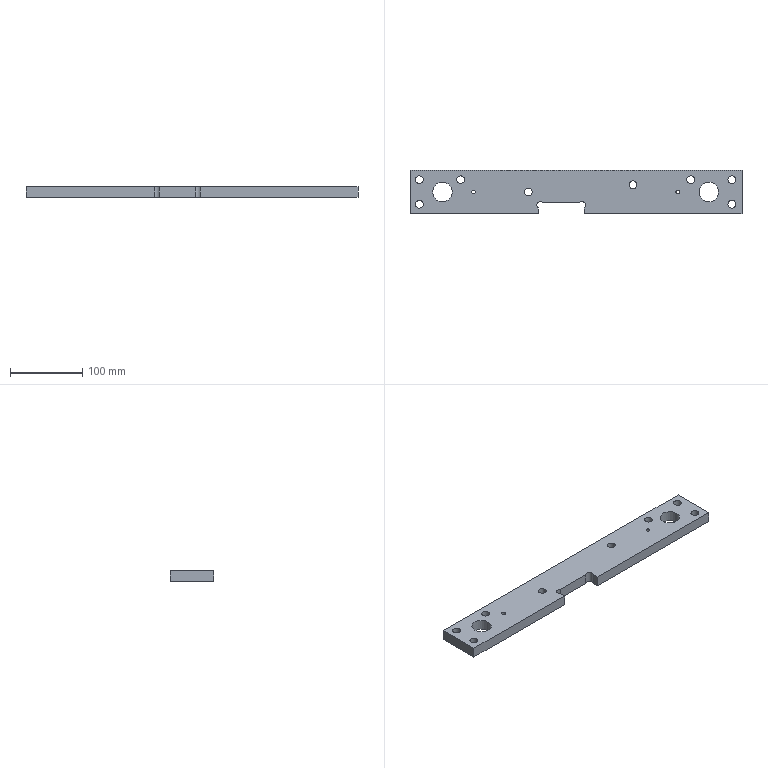Part | NX | features LIN_SOLID_COLOR 2 | 1 solid | 24 faces | box 460 x 60 x 15 mm | volume 369804 mm3 | cylinder 14 | plane 10 | commonest cylinder face diameters 11 x8 5.2 x2 10 x2 27 x2
STEP:
#1=CARTESIAN_POINT('',(530.5,110.,-46.5));
#2=VERTEX_POINT('',#1);
#3=CARTESIAN_POINT('',(353.,110.,-46.5));
#4=VERTEX_POINT('',#3);
#5=CARTESIAN_POINT('',(667.,110.,-46.5));
#6=DIRECTION('',(-1.,0.,0.));
#7=VECTOR('',#6,1000.);
#8=LINE('',#5,#7);
#9=EDGE_CURVE('',#2,#4,#8,.T.);
#10=ORIENTED_EDGE('',*,*,#9,.F.);
#11=CARTESIAN_POINT('',(530.5,110.,-31.5));
#12=VERTEX_POINT('',#11);
#13=CARTESIAN_POINT('',(530.5,110.,-91.5));
#14=DIRECTION('',(0.,0.,1.));
#15=VECTOR('',#14,1000.);
#16=LINE('',#13,#15);
#17=EDGE_CURVE('',#12,#2,#16,.F.);
#18=ORIENTED_EDGE('',*,*,#17,.F.);
#19=CARTESIAN_POINT('',(353.,110.,-31.5));
#20=VERTEX_POINT('',#19);
#21=CARTESIAN_POINT('',(667.,110.,-31.5));
#22=DIRECTION('',(-1.,0.,0.));
#23=VECTOR('',#22,1000.);
#24=LINE('',#21,#23);
#25=EDGE_CURVE('',#20,#12,#24,.F.);
#26=ORIENTED_EDGE('',*,*,#25,.F.);
#27=CARTESIAN_POINT('',(353.,110.,-56.5));
#28=DIRECTION('',(0.,0.,1.));
#29=VECTOR('',#28,1000.);
#30=LINE('',#27,#29);
#31=EDGE_CURVE('',#4,#20,#30,.T.);
#32=ORIENTED_EDGE('',*,*,#31,.F.);
#33=EDGE_LOOP('',(#10,#18,#26,#32));
#34=FACE_BOUND('',#33,.T.);
#35=CARTESIAN_POINT('',(667.,110.,-56.5));
#36=DIRECTION('',(0.,-1.,0.));
#37=DIRECTION('',(0.,0.,1.));
#38=AXIS2_PLACEMENT_3D('',#35,#36,#37);
#39=PLANE('',#38);
#40=ADVANCED_FACE('',(#34),#39,.T.);
#41=CARTESIAN_POINT('',(594.5,110.,-31.5));
#42=VERTEX_POINT('',#41);
#43=CARTESIAN_POINT('',(813.,110.,-31.5));
#44=VERTEX_POINT('',#43);
#45=CARTESIAN_POINT('',(667.,110.,-31.5));
#46=DIRECTION('',(-1.,0.,0.));
#47=VECTOR('',#46,1000.);
#48=LINE('',#45,#47);
#49=EDGE_CURVE('',#42,#44,#48,.F.);
#50=ORIENTED_EDGE('',*,*,#49,.F.);
#51=CARTESIAN_POINT('',(594.5,110.,-46.5));
#52=VERTEX_POINT('',#51);
#53=CARTESIAN_POINT('',(594.5,110.,-91.5));
#54=DIRECTION('',(0.,0.,1.));
#55=VECTOR('',#54,1000.);
#56=LINE('',#53,#55);
#57=EDGE_CURVE('',#52,#42,#56,.T.);
#58=ORIENTED_EDGE('',*,*,#57,.F.);
#59=CARTESIAN_POINT('',(813.,110.,-46.5));
#60=VERTEX_POINT('',#59);
#61=CARTESIAN_POINT('',(667.,110.,-46.5));
#62=DIRECTION('',(-1.,0.,0.));
#63=VECTOR('',#62,1000.);
#64=LINE('',#61,#63);
#65=EDGE_CURVE('',#60,#52,#64,.T.);
#66=ORIENTED_EDGE('',*,*,#65,.F.);
#67=CARTESIAN_POINT('',(813.,110.,-56.5));
#68=DIRECTION('',(0.,0.,1.));
#69=VECTOR('',#68,1000.);
#70=LINE('',#67,#69);
#71=EDGE_CURVE('',#60,#44,#70,.T.);
#72=ORIENTED_EDGE('',*,*,#71,.T.);
#73=EDGE_LOOP('',(#50,#58,#66,#72));
#74=FACE_BOUND('',#73,.T.);
#75=CARTESIAN_POINT('',(667.,110.,-56.5));
#76=DIRECTION('',(0.,-1.,0.));
#77=DIRECTION('',(0.,0.,1.));
#78=AXIS2_PLACEMENT_3D('',#75,#76,#77);
#79=PLANE('',#78);
#80=ADVANCED_FACE('',(#74),#79,.T.);
#81=CARTESIAN_POINT('',(411.5,140.,-31.5));
#82=VERTEX_POINT('',#81);
#83=CARTESIAN_POINT('',(398.,140.,-31.5));
#84=DIRECTION('',(0.,0.,-1.));
#85=DIRECTION('',(1.,0.,0.));
#86=AXIS2_PLACEMENT_3D('',#83,#84,#85);
#87=CIRCLE('',#86,13.5);
#88=EDGE_CURVE('',#82,#82,#87,.F.);
#89=ORIENTED_EDGE('',*,*,#88,.F.);
#90=EDGE_LOOP('',(#89));
#91=FACE_BOUND('',#90,.T.);
#92=CARTESIAN_POINT('',(753.5,140.,-31.5));
#93=VERTEX_POINT('',#92);
#94=CARTESIAN_POINT('',(767.,140.,-31.5));
#95=DIRECTION('',(0.,0.,1.));
#96=DIRECTION('',(-1.,0.,0.));
#97=AXIS2_PLACEMENT_3D('',#94,#95,#96);
#98=CIRCLE('',#97,13.5);
#99=EDGE_CURVE('',#93,#93,#98,.F.);
#100=ORIENTED_EDGE('',*,*,#99,.T.);
#101=EDGE_LOOP('',(#100));
#102=FACE_BOUND('',#101,.T.);
#103=CARTESIAN_POINT('',(371.5,123.,-31.5));
#104=VERTEX_POINT('',#103);
#105=CARTESIAN_POINT('',(366.,123.,-31.5));
#106=DIRECTION('',(0.,0.,1.));
#107=DIRECTION('',(1.,0.,0.));
#108=AXIS2_PLACEMENT_3D('',#105,#106,#107);
#109=CIRCLE('',#108,5.5);
#110=EDGE_CURVE('',#104,#104,#109,.F.);
#111=ORIENTED_EDGE('',*,*,#110,.T.);
#112=EDGE_LOOP('',(#111));
#113=FACE_BOUND('',#112,.T.);
#114=CARTESIAN_POINT('',(522.5,140.,-31.5));
#115=VERTEX_POINT('',#114);
#116=CARTESIAN_POINT('',(517.,140.,-31.5));
#117=DIRECTION('',(0.,0.,1.));
#118=DIRECTION('',(1.,0.,0.));
#119=AXIS2_PLACEMENT_3D('',#116,#117,#118);
#120=CIRCLE('',#119,5.5);
#121=EDGE_CURVE('',#115,#115,#120,.F.);
#122=ORIENTED_EDGE('',*,*,#121,.T.);
#123=EDGE_LOOP('',(#122));
#124=FACE_BOUND('',#123,.T.);
#125=CARTESIAN_POINT('',(747.497,157.,-31.5));
#126=VERTEX_POINT('',#125);
#127=CARTESIAN_POINT('',(741.997,157.,-31.5));
#128=DIRECTION('',(0.,0.,1.));
#129=DIRECTION('',(1.,0.,0.));
#130=AXIS2_PLACEMENT_3D('',#127,#128,#129);
#131=CIRCLE('',#130,5.5);
#132=EDGE_CURVE('',#126,#126,#131,.F.);
#133=ORIENTED_EDGE('',*,*,#132,.T.);
#134=EDGE_LOOP('',(#133));
#135=FACE_BOUND('',#134,.T.);
#136=CARTESIAN_POINT('',(804.5,157.,-31.5));
#137=VERTEX_POINT('',#136);
#138=CARTESIAN_POINT('',(799.,157.,-31.5));
#139=DIRECTION('',(0.,0.,1.));
#140=DIRECTION('',(1.,0.,0.));
#141=AXIS2_PLACEMENT_3D('',#138,#139,#140);
#142=CIRCLE('',#141,5.5);
#143=EDGE_CURVE('',#137,#137,#142,.F.);
#144=ORIENTED_EDGE('',*,*,#143,.T.);
#145=EDGE_LOOP('',(#144));
#146=FACE_BOUND('',#145,.T.);
#147=CARTESIAN_POINT('',(804.5,123.,-31.5));
#148=VERTEX_POINT('',#147);
#149=CARTESIAN_POINT('',(799.,123.,-31.5));
#150=DIRECTION('',(0.,0.,1.));
#151=DIRECTION('',(1.,0.,0.));
#152=AXIS2_PLACEMENT_3D('',#149,#150,#151);
#153=CIRCLE('',#152,5.5);
#154=EDGE_CURVE('',#148,#148,#153,.F.);
#155=ORIENTED_EDGE('',*,*,#154,.T.);
#156=EDGE_LOOP('',(#155));
#157=FACE_BOUND('',#156,.T.);
#158=CARTESIAN_POINT('',(371.5,157.,-31.5));
#159=VERTEX_POINT('',#158);
#160=CARTESIAN_POINT('',(366.,157.,-31.5));
#161=DIRECTION('',(0.,0.,1.));
#162=DIRECTION('',(1.,0.,0.));
#163=AXIS2_PLACEMENT_3D('',#160,#161,#162);
#164=CIRCLE('',#163,5.5);
#165=EDGE_CURVE('',#159,#159,#164,.F.);
#166=ORIENTED_EDGE('',*,*,#165,.T.);
#167=EDGE_LOOP('',(#166));
#168=FACE_BOUND('',#167,.T.);
#169=CARTESIAN_POINT('',(428.503,157.,-31.5));
#170=VERTEX_POINT('',#169);
#171=CARTESIAN_POINT('',(423.003,157.,-31.5));
#172=DIRECTION('',(0.,0.,1.));
#173=DIRECTION('',(1.,0.,0.));
#174=AXIS2_PLACEMENT_3D('',#171,#172,#173);
#175=CIRCLE('',#174,5.5);
#176=EDGE_CURVE('',#170,#170,#175,.F.);
#177=ORIENTED_EDGE('',*,*,#176,.T.);
#178=EDGE_LOOP('',(#177));
#179=FACE_BOUND('',#178,.T.);
#180=CARTESIAN_POINT('',(443.6,140.,-31.5));
#181=VERTEX_POINT('',#180);
#182=CARTESIAN_POINT('',(441.,140.,-31.5));
#183=DIRECTION('',(0.,0.,1.));
#184=DIRECTION('',(1.,0.,0.));
#185=AXIS2_PLACEMENT_3D('',#182,#183,#184);
#186=CIRCLE('',#185,2.6);
#187=EDGE_CURVE('',#181,#181,#186,.T.);
#188=ORIENTED_EDGE('',*,*,#187,.F.);
#189=EDGE_LOOP('',(#188));
#190=FACE_BOUND('',#189,.T.);
#191=CARTESIAN_POINT('',(726.6,140.,-31.5));
#192=VERTEX_POINT('',#191);
#193=CARTESIAN_POINT('',(724.,140.,-31.5));
#194=DIRECTION('',(0.,0.,1.));
#195=DIRECTION('',(1.,0.,0.));
#196=AXIS2_PLACEMENT_3D('',#193,#194,#195);
#197=CIRCLE('',#196,2.6);
#198=EDGE_CURVE('',#192,#192,#197,.T.);
#199=ORIENTED_EDGE('',*,*,#198,.F.);
#200=EDGE_LOOP('',(#199));
#201=FACE_BOUND('',#200,.T.);
#202=CARTESIAN_POINT('',(667.5,150.,-31.5));
#203=VERTEX_POINT('',#202);
#204=CARTESIAN_POINT('',(662.,150.,-31.5));
#205=DIRECTION('',(0.,0.,1.));
#206=DIRECTION('',(1.,0.,0.));
#207=AXIS2_PLACEMENT_3D('',#204,#205,#206);
#208=CIRCLE('',#207,5.5);
#209=EDGE_CURVE('',#203,#203,#208,.T.);
#210=ORIENTED_EDGE('',*,*,#209,.F.);
#211=EDGE_LOOP('',(#210));
#212=FACE_BOUND('',#211,.T.);
#213=ORIENTED_EDGE('',*,*,#25,.T.);
#214=CARTESIAN_POINT('',(530.5,117.961,-31.5));
#215=VERTEX_POINT('',#214);
#216=CARTESIAN_POINT('',(530.5,140.,-31.5));
#217=DIRECTION('',(0.,1.,0.));
#218=VECTOR('',#217,1000.);
#219=LINE('',#216,#218);
#220=EDGE_CURVE('',#12,#215,#219,.T.);
#221=ORIENTED_EDGE('',*,*,#220,.T.);
#222=CARTESIAN_POINT('',(537.539,125.,-31.5));
#223=VERTEX_POINT('',#222);
#224=CARTESIAN_POINT('',(533.682,121.818,-31.5));
#225=DIRECTION('',(0.,0.,1.));
#226=DIRECTION('',(1.,0.,0.));
#227=AXIS2_PLACEMENT_3D('',#224,#225,#226);
#228=CIRCLE('',#227,5.);
#229=EDGE_CURVE('',#223,#215,#228,.T.);
#230=ORIENTED_EDGE('',*,*,#229,.F.);
#231=CARTESIAN_POINT('',(587.461,125.,-31.5));
#232=VERTEX_POINT('',#231);
#233=CARTESIAN_POINT('',(667.,125.,-31.5));
#234=DIRECTION('',(1.,0.,0.));
#235=VECTOR('',#234,1000.);
#236=LINE('',#233,#235);
#237=EDGE_CURVE('',#223,#232,#236,.T.);
#238=ORIENTED_EDGE('',*,*,#237,.T.);
#239=CARTESIAN_POINT('',(594.5,117.961,-31.5));
#240=VERTEX_POINT('',#239);
#241=CARTESIAN_POINT('',(591.318,121.818,-31.5));
#242=DIRECTION('',(0.,0.,1.));
#243=DIRECTION('',(1.,0.,0.));
#244=AXIS2_PLACEMENT_3D('',#241,#242,#243);
#245=CIRCLE('',#244,5.);
#246=EDGE_CURVE('',#232,#240,#245,.F.);
#247=ORIENTED_EDGE('',*,*,#246,.T.);
#248=CARTESIAN_POINT('',(594.5,140.,-31.5));
#249=DIRECTION('',(0.,-1.,0.));
#250=VECTOR('',#249,1000.);
#251=LINE('',#248,#250);
#252=EDGE_CURVE('',#42,#240,#251,.F.);
#253=ORIENTED_EDGE('',*,*,#252,.F.);
#254=ORIENTED_EDGE('',*,*,#49,.T.);
#255=CARTESIAN_POINT('',(813.,170.,-31.5));
#256=VERTEX_POINT('',#255);
#257=CARTESIAN_POINT('',(813.,30.,-31.5));
#258=DIRECTION('',(0.,-1.,0.));
#259=VECTOR('',#258,1000.);
#260=LINE('',#257,#259);
#261=EDGE_CURVE('',#256,#44,#260,.T.);
#262=ORIENTED_EDGE('',*,*,#261,.F.);
#263=CARTESIAN_POINT('',(353.,170.,-31.5));
#264=VERTEX_POINT('',#263);
#265=CARTESIAN_POINT('',(667.,170.,-31.5));
#266=DIRECTION('',(1.,0.,0.));
#267=VECTOR('',#266,1000.);
#268=LINE('',#265,#267);
#269=EDGE_CURVE('',#256,#264,#268,.F.);
#270=ORIENTED_EDGE('',*,*,#269,.T.);
#271=CARTESIAN_POINT('',(353.,30.,-31.5));
#272=DIRECTION('',(0.,-1.,0.));
#273=VECTOR('',#272,1000.);
#274=LINE('',#271,#273);
#275=EDGE_CURVE('',#264,#20,#274,.T.);
#276=ORIENTED_EDGE('',*,*,#275,.T.);
#277=EDGE_LOOP('',(#213,#221,#230,#238,#247,#253,#254,#262,#270,#276));
#278=FACE_BOUND('',#277,.T.);
#279=CARTESIAN_POINT('',(667.,140.,-31.5));
#280=DIRECTION('',(0.,0.,1.));
#281=DIRECTION('',(-1.,0.,0.));
#282=AXIS2_PLACEMENT_3D('',#279,#280,#281);
#283=PLANE('',#282);
#284=ADVANCED_FACE('',(#91,#102,#113,#124,#135,#146,#157,#168,#179,#190,#201,#212,#278),#283,.T.);
#285=CARTESIAN_POINT('',(438.4,140.,-46.5));
#286=VERTEX_POINT('',#285);
#287=CARTESIAN_POINT('',(441.,140.,-46.5));
#288=DIRECTION('',(0.,0.,-1.));
#289=DIRECTION('',(-1.,0.,0.));
#290=AXIS2_PLACEMENT_3D('',#287,#288,#289);
#291=CIRCLE('',#290,2.6);
#292=EDGE_CURVE('',#286,#286,#291,.F.);
#293=ORIENTED_EDGE('',*,*,#292,.T.);
#294=EDGE_LOOP('',(#293));
#295=FACE_BOUND('',#294,.T.);
#296=CARTESIAN_POINT('',(384.5,140.,-46.5));
#297=VERTEX_POINT('',#296);
#298=CARTESIAN_POINT('',(398.,140.,-46.5));
#299=DIRECTION('',(0.,0.,-1.));
#300=DIRECTION('',(-1.,0.,0.));
#301=AXIS2_PLACEMENT_3D('',#298,#299,#300);
#302=CIRCLE('',#301,13.5);
#303=EDGE_CURVE('',#297,#297,#302,.T.);
#304=ORIENTED_EDGE('',*,*,#303,.F.);
#305=EDGE_LOOP('',(#304));
#306=FACE_BOUND('',#305,.T.);
#307=CARTESIAN_POINT('',(753.5,140.,-46.5));
#308=VERTEX_POINT('',#307);
#309=CARTESIAN_POINT('',(767.,140.,-46.5));
#310=DIRECTION('',(0.,0.,-1.));
#311=DIRECTION('',(-1.,0.,0.));
#312=AXIS2_PLACEMENT_3D('',#309,#310,#311);
#313=CIRCLE('',#312,13.5);
#314=EDGE_CURVE('',#308,#308,#313,.F.);
#315=ORIENTED_EDGE('',*,*,#314,.T.);
#316=EDGE_LOOP('',(#315));
#317=FACE_BOUND('',#316,.T.);
#318=CARTESIAN_POINT('',(360.5,123.,-46.5));
#319=VERTEX_POINT('',#318);
#320=CARTESIAN_POINT('',(366.,123.,-46.5));
#321=DIRECTION('',(0.,0.,-1.));
#322=DIRECTION('',(-1.,0.,0.));
#323=AXIS2_PLACEMENT_3D('',#320,#321,#322);
#324=CIRCLE('',#323,5.5);
#325=EDGE_CURVE('',#319,#319,#324,.F.);
#326=ORIENTED_EDGE('',*,*,#325,.T.);
#327=EDGE_LOOP('',(#326));
#328=FACE_BOUND('',#327,.T.);
#329=CARTESIAN_POINT('',(511.5,140.,-46.5));
#330=VERTEX_POINT('',#329);
#331=CARTESIAN_POINT('',(517.,140.,-46.5));
#332=DIRECTION('',(0.,0.,-1.));
#333=DIRECTION('',(-1.,0.,0.));
#334=AXIS2_PLACEMENT_3D('',#331,#332,#333);
#335=CIRCLE('',#334,5.5);
#336=EDGE_CURVE('',#330,#330,#335,.F.);
#337=ORIENTED_EDGE('',*,*,#336,.T.);
#338=EDGE_LOOP('',(#337));
#339=FACE_BOUND('',#338,.T.);
#340=CARTESIAN_POINT('',(736.497,157.,-46.5));
#341=VERTEX_POINT('',#340);
#342=CARTESIAN_POINT('',(741.997,157.,-46.5));
#343=DIRECTION('',(0.,0.,-1.));
#344=DIRECTION('',(-1.,0.,0.));
#345=AXIS2_PLACEMENT_3D('',#342,#343,#344);
#346=CIRCLE('',#345,5.5);
#347=EDGE_CURVE('',#341,#341,#346,.F.);
#348=ORIENTED_EDGE('',*,*,#347,.T.);
#349=EDGE_LOOP('',(#348));
#350=FACE_BOUND('',#349,.T.);
#351=CARTESIAN_POINT('',(793.5,157.,-46.5));
#352=VERTEX_POINT('',#351);
#353=CARTESIAN_POINT('',(799.,157.,-46.5));
#354=DIRECTION('',(0.,0.,-1.));
#355=DIRECTION('',(-1.,0.,0.));
#356=AXIS2_PLACEMENT_3D('',#353,#354,#355);
#357=CIRCLE('',#356,5.5);
#358=EDGE_CURVE('',#352,#352,#357,.F.);
#359=ORIENTED_EDGE('',*,*,#358,.T.);
#360=EDGE_LOOP('',(#359));
#361=FACE_BOUND('',#360,.T.);
#362=CARTESIAN_POINT('',(793.5,123.,-46.5));
#363=VERTEX_POINT('',#362);
#364=CARTESIAN_POINT('',(799.,123.,-46.5));
#365=DIRECTION('',(0.,0.,-1.));
#366=DIRECTION('',(-1.,0.,0.));
#367=AXIS2_PLACEMENT_3D('',#364,#365,#366);
#368=CIRCLE('',#367,5.5);
#369=EDGE_CURVE('',#363,#363,#368,.F.);
#370=ORIENTED_EDGE('',*,*,#369,.T.);
#371=EDGE_LOOP('',(#370));
#372=FACE_BOUND('',#371,.T.);
#373=CARTESIAN_POINT('',(360.5,157.,-46.5));
#374=VERTEX_POINT('',#373);
#375=CARTESIAN_POINT('',(366.,157.,-46.5));
#376=DIRECTION('',(0.,0.,-1.));
#377=DIRECTION('',(-1.,0.,0.));
#378=AXIS2_PLACEMENT_3D('',#375,#376,#377);
#379=CIRCLE('',#378,5.5);
#380=EDGE_CURVE('',#374,#374,#379,.F.);
#381=ORIENTED_EDGE('',*,*,#380,.T.);
#382=EDGE_LOOP('',(#381));
#383=FACE_BOUND('',#382,.T.);
#384=CARTESIAN_POINT('',(417.503,157.,-46.5));
#385=VERTEX_POINT('',#384);
#386=CARTESIAN_POINT('',(423.003,157.,-46.5));
#387=DIRECTION('',(0.,0.,-1.));
#388=DIRECTION('',(-1.,0.,0.));
#389=AXIS2_PLACEMENT_3D('',#386,#387,#388);
#390=CIRCLE('',#389,5.5);
#391=EDGE_CURVE('',#385,#385,#390,.F.);
#392=ORIENTED_EDGE('',*,*,#391,.T.);
#393=EDGE_LOOP('',(#392));
#394=FACE_BOUND('',#393,.T.);
#395=CARTESIAN_POINT('',(721.4,140.,-46.5));
#396=VERTEX_POINT('',#395);
#397=CARTESIAN_POINT('',(724.,140.,-46.5));
#398=DIRECTION('',(0.,0.,-1.));
#399=DIRECTION('',(-1.,0.,0.));
#400=AXIS2_PLACEMENT_3D('',#397,#398,#399);
#401=CIRCLE('',#400,2.6);
#402=EDGE_CURVE('',#396,#396,#401,.F.);
#403=ORIENTED_EDGE('',*,*,#402,.T.);
#404=EDGE_LOOP('',(#403));
#405=FACE_BOUND('',#404,.T.);
#406=CARTESIAN_POINT('',(656.5,150.,-46.5));
#407=VERTEX_POINT('',#406);
#408=CARTESIAN_POINT('',(662.,150.,-46.5));
#409=DIRECTION('',(0.,0.,-1.));
#410=DIRECTION('',(-1.,0.,0.));
#411=AXIS2_PLACEMENT_3D('',#408,#409,#410);
#412=CIRCLE('',#411,5.5);
#413=EDGE_CURVE('',#407,#407,#412,.T.);
#414=ORIENTED_EDGE('',*,*,#413,.F.);
#415=EDGE_LOOP('',(#414));
#416=FACE_BOUND('',#415,.T.);
#417=CARTESIAN_POINT('',(537.539,125.,-46.5));
#418=VERTEX_POINT('',#417);
#419=CARTESIAN_POINT('',(530.5,117.961,-46.5));
#420=VERTEX_POINT('',#419);
#421=CARTESIAN_POINT('',(533.682,121.818,-46.5));
#422=DIRECTION('',(0.,0.,-1.));
#423=DIRECTION('',(-1.,0.,0.));
#424=AXIS2_PLACEMENT_3D('',#421,#422,#423);
#425=CIRCLE('',#424,5.);
#426=EDGE_CURVE('',#418,#420,#425,.F.);
#427=ORIENTED_EDGE('',*,*,#426,.T.);
#428=CARTESIAN_POINT('',(530.5,140.,-46.5));
#429=DIRECTION('',(0.,-1.,0.));
#430=VECTOR('',#429,1000.);
#431=LINE('',#428,#430);
#432=EDGE_CURVE('',#2,#420,#431,.F.);
#433=ORIENTED_EDGE('',*,*,#432,.F.);
#434=ORIENTED_EDGE('',*,*,#9,.T.);
#435=CARTESIAN_POINT('',(353.,170.,-46.5));
#436=VERTEX_POINT('',#435);
#437=CARTESIAN_POINT('',(353.,140.,-46.5));
#438=DIRECTION('',(0.,1.,0.));
#439=VECTOR('',#438,1000.);
#440=LINE('',#437,#439);
#441=EDGE_CURVE('',#4,#436,#440,.T.);
#442=ORIENTED_EDGE('',*,*,#441,.T.);
#443=CARTESIAN_POINT('',(813.,170.,-46.5));
#444=VERTEX_POINT('',#443);
#445=CARTESIAN_POINT('',(667.,170.,-46.5));
#446=DIRECTION('',(1.,0.,0.));
#447=VECTOR('',#446,1000.);
#448=LINE('',#445,#447);
#449=EDGE_CURVE('',#436,#444,#448,.T.);
#450=ORIENTED_EDGE('',*,*,#449,.T.);
#451=CARTESIAN_POINT('',(813.,30.,-46.5));
#452=DIRECTION('',(0.,1.,0.));
#453=VECTOR('',#452,1000.);
#454=LINE('',#451,#453);
#455=EDGE_CURVE('',#60,#444,#454,.T.);
#456=ORIENTED_EDGE('',*,*,#455,.F.);
#457=ORIENTED_EDGE('',*,*,#65,.T.);
#458=CARTESIAN_POINT('',(594.5,117.961,-46.5));
#459=VERTEX_POINT('',#458);
#460=CARTESIAN_POINT('',(594.5,140.,-46.5));
#461=DIRECTION('',(0.,1.,0.));
#462=VECTOR('',#461,1000.);
#463=LINE('',#460,#462);
#464=EDGE_CURVE('',#459,#52,#463,.F.);
#465=ORIENTED_EDGE('',*,*,#464,.F.);
#466=CARTESIAN_POINT('',(587.461,125.,-46.5));
#467=VERTEX_POINT('',#466);
#468=CARTESIAN_POINT('',(591.318,121.818,-46.5));
#469=DIRECTION('',(0.,0.,-1.));
#470=DIRECTION('',(-1.,0.,0.));
#471=AXIS2_PLACEMENT_3D('',#468,#469,#470);
#472=CIRCLE('',#471,5.);
#473=EDGE_CURVE('',#467,#459,#472,.T.);
#474=ORIENTED_EDGE('',*,*,#473,.F.);
#475=CARTESIAN_POINT('',(667.,125.,-46.5));
#476=DIRECTION('',(-1.,0.,0.));
#477=VECTOR('',#476,1000.);
#478=LINE('',#475,#477);
#479=EDGE_CURVE('',#467,#418,#478,.T.);
#480=ORIENTED_EDGE('',*,*,#479,.T.);
#481=EDGE_LOOP('',(#427,#433,#434,#442,#450,#456,#457,#465,#474,#480));
#482=FACE_BOUND('',#481,.T.);
#483=CARTESIAN_POINT('',(667.,140.,-46.5));
#484=DIRECTION('',(0.,0.,-1.));
#485=DIRECTION('',(1.,0.,0.));
#486=AXIS2_PLACEMENT_3D('',#483,#484,#485);
#487=PLANE('',#486);
#488=ADVANCED_FACE('',(#295,#306,#317,#328,#339,#350,#361,#372,#383,#394,#405,#416,#482),#487,.T.);
#489=ORIENTED_EDGE('',*,*,#209,.T.);
#490=EDGE_LOOP('',(#489));
#491=FACE_BOUND('',#490,.T.);
#492=ORIENTED_EDGE('',*,*,#413,.T.);
#493=EDGE_LOOP('',(#492));
#494=FACE_BOUND('',#493,.T.);
#495=CARTESIAN_POINT('',(662.,150.,-31.4));
#496=DIRECTION('',(0.,0.,-1.));
#497=DIRECTION('',(1.,0.,0.));
#498=AXIS2_PLACEMENT_3D('',#495,#496,#497);
#499=CYLINDRICAL_SURFACE('',#498,5.5);
#500=ADVANCED_FACE('',(#491,#494),#499,.F.);
#501=ORIENTED_EDGE('',*,*,#88,.T.);
#502=EDGE_LOOP('',(#501));
#503=FACE_BOUND('',#502,.T.);
#504=ORIENTED_EDGE('',*,*,#303,.T.);
#505=EDGE_LOOP('',(#504));
#506=FACE_BOUND('',#505,.T.);
#507=CARTESIAN_POINT('',(398.,140.,-1.));
#508=DIRECTION('',(0.,0.,-1.));
#509=DIRECTION('',(-1.,0.,0.));
#510=AXIS2_PLACEMENT_3D('',#507,#508,#509);
#511=CYLINDRICAL_SURFACE('',#510,13.5);
#512=ADVANCED_FACE('',(#503,#506),#511,.F.);
#513=ORIENTED_EDGE('',*,*,#99,.F.);
#514=EDGE_LOOP('',(#513));
#515=FACE_BOUND('',#514,.T.);
#516=ORIENTED_EDGE('',*,*,#314,.F.);
#517=EDGE_LOOP('',(#516));
#518=FACE_BOUND('',#517,.T.);
#519=CARTESIAN_POINT('',(767.,140.,-1.));
#520=DIRECTION('',(0.,0.,-1.));
#521=DIRECTION('',(1.,0.,0.));
#522=AXIS2_PLACEMENT_3D('',#519,#520,#521);
#523=CYLINDRICAL_SURFACE('',#522,13.5);
#524=ADVANCED_FACE('',(#515,#518),#523,.F.);
#525=CARTESIAN_POINT('',(813.,170.,12.5));
#526=DIRECTION('',(0.,0.,1.));
#527=VECTOR('',#526,1000.);
#528=LINE('',#525,#527);
#529=EDGE_CURVE('',#444,#256,#528,.T.);
#530=ORIENTED_EDGE('',*,*,#529,.T.);
#531=ORIENTED_EDGE('',*,*,#261,.T.);
#532=ORIENTED_EDGE('',*,*,#71,.F.);
#533=ORIENTED_EDGE('',*,*,#455,.T.);
#534=EDGE_LOOP('',(#530,#531,#532,#533));
#535=FACE_BOUND('',#534,.T.);
#536=CARTESIAN_POINT('',(813.,30.,12.5));
#537=DIRECTION('',(1.,0.,0.));
#538=DIRECTION('',(0.,0.,-1.));
#539=AXIS2_PLACEMENT_3D('',#536,#537,#538);
#540=PLANE('',#539);
#541=ADVANCED_FACE('',(#535),#540,.T.);
#542=CARTESIAN_POINT('',(353.,170.,25.));
#543=DIRECTION('',(0.,0.,1.));
#544=VECTOR('',#543,1000.);
#545=LINE('',#542,#544);
#546=EDGE_CURVE('',#436,#264,#545,.T.);
#547=ORIENTED_EDGE('',*,*,#546,.F.);
#548=ORIENTED_EDGE('',*,*,#441,.F.);
#549=ORIENTED_EDGE('',*,*,#31,.T.);
#550=ORIENTED_EDGE('',*,*,#275,.F.);
#551=EDGE_LOOP('',(#547,#548,#549,#550));
#552=FACE_BOUND('',#551,.T.);
#553=CARTESIAN_POINT('',(353.,30.,25.));
#554=DIRECTION('',(-1.,0.,0.));
#555=DIRECTION('',(0.,0.,1.));
#556=AXIS2_PLACEMENT_3D('',#553,#554,#555);
#557=PLANE('',#556);
#558=ADVANCED_FACE('',(#552),#557,.T.);
#559=ORIENTED_EDGE('',*,*,#269,.F.);
#560=ORIENTED_EDGE('',*,*,#529,.F.);
#561=ORIENTED_EDGE('',*,*,#449,.F.);
#562=ORIENTED_EDGE('',*,*,#546,.T.);
#563=EDGE_LOOP('',(#559,#560,#561,#562));
#564=FACE_BOUND('',#563,.T.);
#565=CARTESIAN_POINT('',(667.,170.,-56.5));
#566=DIRECTION('',(0.,1.,0.));
#567=DIRECTION('',(0.,0.,-1.));
#568=AXIS2_PLACEMENT_3D('',#565,#566,#567);
#569=PLANE('',#568);
#570=ADVANCED_FACE('',(#564),#569,.T.);
#571=ORIENTED_EDGE('',*,*,#110,.F.);
#572=EDGE_LOOP('',(#571));
#573=FACE_BOUND('',#572,.T.);
#574=ORIENTED_EDGE('',*,*,#325,.F.);
#575=EDGE_LOOP('',(#574));
#576=FACE_BOUND('',#575,.T.);
#577=CARTESIAN_POINT('',(366.,123.,-31.4));
#578=DIRECTION('',(0.,0.,-1.));
#579=DIRECTION('',(1.,0.,0.));
#580=AXIS2_PLACEMENT_3D('',#577,#578,#579);
#581=CYLINDRICAL_SURFACE('',#580,5.5);
#582=ADVANCED_FACE('',(#573,#576),#581,.F.);
#583=ORIENTED_EDGE('',*,*,#121,.F.);
#584=EDGE_LOOP('',(#583));
#585=FACE_BOUND('',#584,.T.);
#586=ORIENTED_EDGE('',*,*,#336,.F.);
#587=EDGE_LOOP('',(#586));
#588=FACE_BOUND('',#587,.T.);
#589=CARTESIAN_POINT('',(517.,140.,-31.4));
#590=DIRECTION('',(0.,0.,-1.));
#591=DIRECTION('',(1.,0.,0.));
#592=AXIS2_PLACEMENT_3D('',#589,#590,#591);
#593=CYLINDRICAL_SURFACE('',#592,5.5);
#594=ADVANCED_FACE('',(#585,#588),#593,.F.);
#595=ORIENTED_EDGE('',*,*,#132,.F.);
#596=EDGE_LOOP('',(#595));
#597=FACE_BOUND('',#596,.T.);
#598=ORIENTED_EDGE('',*,*,#347,.F.);
#599=EDGE_LOOP('',(#598));
#600=FACE_BOUND('',#599,.T.);
#601=CARTESIAN_POINT('',(741.997,157.,-31.4));
#602=DIRECTION('',(0.,0.,-1.));
#603=DIRECTION('',(1.,0.,0.));
#604=AXIS2_PLACEMENT_3D('',#601,#602,#603);
#605=CYLINDRICAL_SURFACE('',#604,5.5);
#606=ADVANCED_FACE('',(#597,#600),#605,.F.);
#607=ORIENTED_EDGE('',*,*,#143,.F.);
#608=EDGE_LOOP('',(#607));
#609=FACE_BOUND('',#608,.T.);
#610=ORIENTED_EDGE('',*,*,#358,.F.);
#611=EDGE_LOOP('',(#610));
#612=FACE_BOUND('',#611,.T.);
#613=CARTESIAN_POINT('',(799.,157.,-31.4));
#614=DIRECTION('',(0.,0.,-1.));
#615=DIRECTION('',(1.,0.,0.));
#616=AXIS2_PLACEMENT_3D('',#613,#614,#615);
#617=CYLINDRICAL_SURFACE('',#616,5.5);
#618=ADVANCED_FACE('',(#609,#612),#617,.F.);
#619=ORIENTED_EDGE('',*,*,#154,.F.);
#620=EDGE_LOOP('',(#619));
#621=FACE_BOUND('',#620,.T.);
#622=ORIENTED_EDGE('',*,*,#369,.F.);
#623=EDGE_LOOP('',(#622));
#624=FACE_BOUND('',#623,.T.);
#625=CARTESIAN_POINT('',(799.,123.,-31.4));
#626=DIRECTION('',(0.,0.,-1.));
#627=DIRECTION('',(1.,0.,0.));
#628=AXIS2_PLACEMENT_3D('',#625,#626,#627);
#629=CYLINDRICAL_SURFACE('',#628,5.5);
#630=ADVANCED_FACE('',(#621,#624),#629,.F.);
#631=ORIENTED_EDGE('',*,*,#165,.F.);
#632=EDGE_LOOP('',(#631));
#633=FACE_BOUND('',#632,.T.);
#634=ORIENTED_EDGE('',*,*,#380,.F.);
#635=EDGE_LOOP('',(#634));
#636=FACE_BOUND('',#635,.T.);
#637=CARTESIAN_POINT('',(366.,157.,-31.4));
#638=DIRECTION('',(0.,0.,-1.));
#639=DIRECTION('',(1.,0.,0.));
#640=AXIS2_PLACEMENT_3D('',#637,#638,#639);
#641=CYLINDRICAL_SURFACE('',#640,5.5);
#642=ADVANCED_FACE('',(#633,#636),#641,.F.);
#643=ORIENTED_EDGE('',*,*,#176,.F.);
#644=EDGE_LOOP('',(#643));
#645=FACE_BOUND('',#644,.T.);
#646=ORIENTED_EDGE('',*,*,#391,.F.);
#647=EDGE_LOOP('',(#646));
#648=FACE_BOUND('',#647,.T.);
#649=CARTESIAN_POINT('',(423.003,157.,-31.4));
#650=DIRECTION('',(0.,0.,-1.));
#651=DIRECTION('',(1.,0.,0.));
#652=AXIS2_PLACEMENT_3D('',#649,#650,#651);
#653=CYLINDRICAL_SURFACE('',#652,5.5);
#654=ADVANCED_FACE('',(#645,#648),#653,.F.);
#655=ORIENTED_EDGE('',*,*,#292,.F.);
#656=EDGE_LOOP('',(#655));
#657=FACE_BOUND('',#656,.T.);
#658=ORIENTED_EDGE('',*,*,#187,.T.);
#659=EDGE_LOOP('',(#658));
#660=FACE_BOUND('',#659,.T.);
#661=CARTESIAN_POINT('',(441.,140.,-31.4));
#662=DIRECTION('',(0.,0.,-1.));
#663=DIRECTION('',(1.,0.,0.));
#664=AXIS2_PLACEMENT_3D('',#661,#662,#663);
#665=CYLINDRICAL_SURFACE('',#664,2.6);
#666=ADVANCED_FACE('',(#657,#660),#665,.F.);
#667=ORIENTED_EDGE('',*,*,#402,.F.);
#668=EDGE_LOOP('',(#667));
#669=FACE_BOUND('',#668,.T.);
#670=ORIENTED_EDGE('',*,*,#198,.T.);
#671=EDGE_LOOP('',(#670));
#672=FACE_BOUND('',#671,.T.);
#673=CARTESIAN_POINT('',(724.,140.,-31.4));
#674=DIRECTION('',(0.,0.,-1.));
#675=DIRECTION('',(1.,0.,0.));
#676=AXIS2_PLACEMENT_3D('',#673,#674,#675);
#677=CYLINDRICAL_SURFACE('',#676,2.6);
#678=ADVANCED_FACE('',(#669,#672),#677,.F.);
#679=ORIENTED_EDGE('',*,*,#220,.F.);
#680=ORIENTED_EDGE('',*,*,#17,.T.);
#681=ORIENTED_EDGE('',*,*,#432,.T.);
#682=CARTESIAN_POINT('',(530.5,117.961,-91.5));
#683=DIRECTION('',(0.,0.,1.));
#684=VECTOR('',#683,1000.);
#685=LINE('',#682,#684);
#686=EDGE_CURVE('',#420,#215,#685,.T.);
#687=ORIENTED_EDGE('',*,*,#686,.T.);
#688=EDGE_LOOP('',(#679,#680,#681,#687));
#689=FACE_BOUND('',#688,.T.);
#690=CARTESIAN_POINT('',(530.5,110.,-91.5));
#691=DIRECTION('',(1.,0.,0.));
#692=DIRECTION('',(0.,0.,-1.));
#693=AXIS2_PLACEMENT_3D('',#690,#691,#692);
#694=PLANE('',#693);
#695=ADVANCED_FACE('',(#689),#694,.T.);
#696=ORIENTED_EDGE('',*,*,#229,.T.);
#697=ORIENTED_EDGE('',*,*,#686,.F.);
#698=ORIENTED_EDGE('',*,*,#426,.F.);
#699=CARTESIAN_POINT('',(537.539,125.,-91.5));
#700=DIRECTION('',(0.,0.,1.));
#701=VECTOR('',#700,1000.);
#702=LINE('',#699,#701);
#703=EDGE_CURVE('',#418,#223,#702,.T.);
#704=ORIENTED_EDGE('',*,*,#703,.T.);
#705=EDGE_LOOP('',(#696,#697,#698,#704));
#706=FACE_BOUND('',#705,.T.);
#707=CARTESIAN_POINT('',(533.682,121.818,-91.5));
#708=DIRECTION('',(0.,0.,1.));
#709=DIRECTION('',(1.,0.,0.));
#710=AXIS2_PLACEMENT_3D('',#707,#708,#709);
#711=CYLINDRICAL_SURFACE('',#710,5.);
#712=ADVANCED_FACE('',(#706),#711,.F.);
#713=ORIENTED_EDGE('',*,*,#237,.F.);
#714=ORIENTED_EDGE('',*,*,#703,.F.);
#715=ORIENTED_EDGE('',*,*,#479,.F.);
#716=CARTESIAN_POINT('',(587.461,125.,-91.5));
#717=DIRECTION('',(0.,0.,1.));
#718=VECTOR('',#717,1000.);
#719=LINE('',#716,#718);
#720=EDGE_CURVE('',#467,#232,#719,.T.);
#721=ORIENTED_EDGE('',*,*,#720,.T.);
#722=EDGE_LOOP('',(#713,#714,#715,#721));
#723=FACE_BOUND('',#722,.T.);
#724=CARTESIAN_POINT('',(537.539,125.,-91.5));
#725=DIRECTION('',(0.,-1.,0.));
#726=DIRECTION('',(0.,0.,-1.));
#727=AXIS2_PLACEMENT_3D('',#724,#725,#726);
#728=PLANE('',#727);
#729=ADVANCED_FACE('',(#723),#728,.T.);
#730=ORIENTED_EDGE('',*,*,#246,.F.);
#731=ORIENTED_EDGE('',*,*,#720,.F.);
#732=ORIENTED_EDGE('',*,*,#473,.T.);
#733=CARTESIAN_POINT('',(594.5,117.961,-91.5));
#734=DIRECTION('',(0.,0.,1.));
#735=VECTOR('',#734,1000.);
#736=LINE('',#733,#735);
#737=EDGE_CURVE('',#459,#240,#736,.T.);
#738=ORIENTED_EDGE('',*,*,#737,.T.);
#739=EDGE_LOOP('',(#730,#731,#732,#738));
#740=FACE_BOUND('',#739,.T.);
#741=CARTESIAN_POINT('',(591.318,121.818,-91.5));
#742=DIRECTION('',(0.,0.,1.));
#743=DIRECTION('',(1.,0.,0.));
#744=AXIS2_PLACEMENT_3D('',#741,#742,#743);
#745=CYLINDRICAL_SURFACE('',#744,5.);
#746=ADVANCED_FACE('',(#740),#745,.F.);
#747=ORIENTED_EDGE('',*,*,#252,.T.);
#748=ORIENTED_EDGE('',*,*,#737,.F.);
#749=ORIENTED_EDGE('',*,*,#464,.T.);
#750=ORIENTED_EDGE('',*,*,#57,.T.);
#751=EDGE_LOOP('',(#747,#748,#749,#750));
#752=FACE_BOUND('',#751,.T.);
#753=CARTESIAN_POINT('',(594.5,114.961,-91.5));
#754=DIRECTION('',(-1.,0.,0.));
#755=DIRECTION('',(0.,0.,1.));
#756=AXIS2_PLACEMENT_3D('',#753,#754,#755);
#757=PLANE('',#756);
#758=ADVANCED_FACE('',(#752),#757,.T.);
#759=CLOSED_SHELL('',(#40,#80,#284,#488,#500,#512,#524,#541,#558,#570,#582,#594,#606,#618,#630,#642,#654,#666,#678,#695,#712,#729,#746,#758));
#760=MANIFOLD_SOLID_BREP('',#759);
#761=(LENGTH_UNIT()NAMED_UNIT(*)SI_UNIT(.MILLI.,.METRE.));
#762=UNCERTAINTY_MEASURE_WITH_UNIT(LENGTH_MEASURE(0.00001),#761,'','');
#763=(NAMED_UNIT(*)PLANE_ANGLE_UNIT()SI_UNIT($,.RADIAN.));
#764=(NAMED_UNIT(*)SI_UNIT($,.STERADIAN.)SOLID_ANGLE_UNIT());
#765=(GEOMETRIC_REPRESENTATION_CONTEXT(3)GLOBAL_UNCERTAINTY_ASSIGNED_CONTEXT((#762))GLOBAL_UNIT_ASSIGNED_CONTEXT((#761,#763,#764))REPRESENTATION_CONTEXT('',''));
#766=ADVANCED_BREP_SHAPE_REPRESENTATION('',(#760),#765);